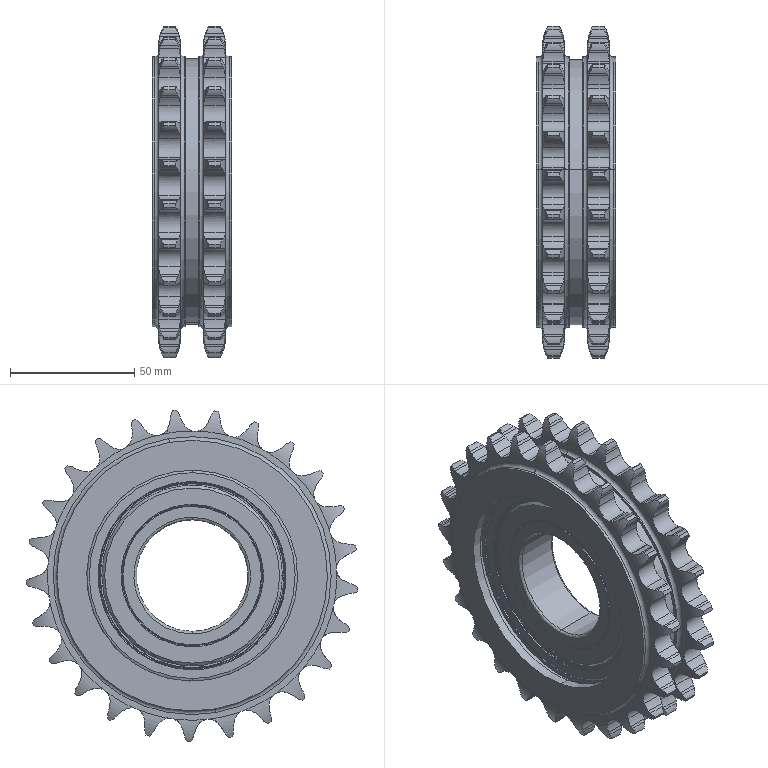Part | SolidWorks | 2 solids | 699 faces | box 32.003 x 133.797 x 133.698 mm | volume 230704 mm3 | cylinder 368 | plane 123 | torus 112 | spline 56 | cone 40 | commonest cylinder face diameters 14.66 x104 26.567 x104 10.311 x64 134 x50 109 x8 85 x6